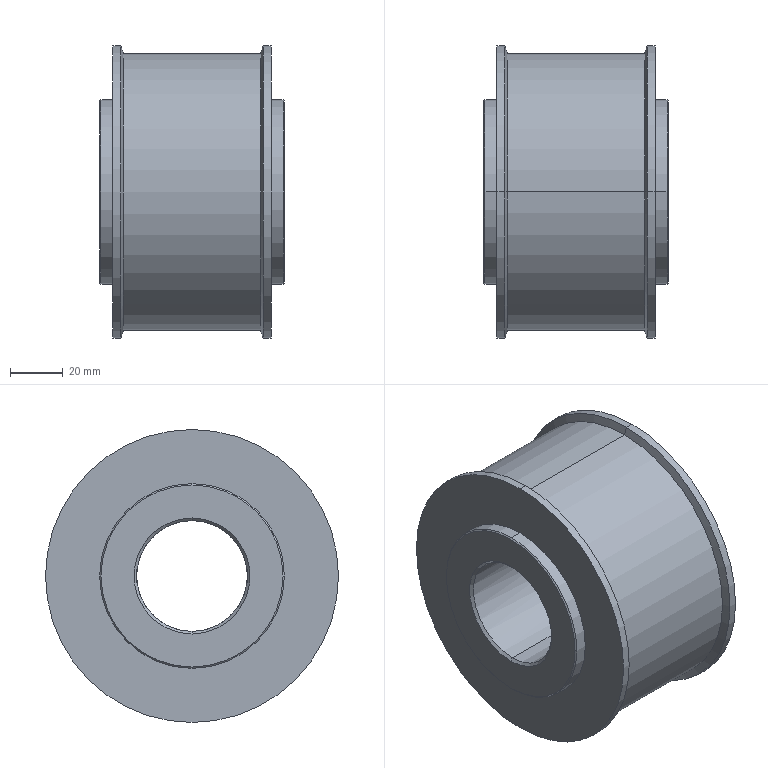Part | SolidWorks | features BaseBody 1 | 1 solid | 36 faces | box 70 x 111 x 111 mm | volume 426027 mm3 | cylinder 16 | cone 14 | plane 6 | commonest cylinder face diameters 70 x4 111 x4 42 x2 52 x2 62 x2 105 x2
STEP:
#1=CARTESIAN_POINT('',(-26.,0.,-52.5));
#2=VERTEX_POINT('',#1);
#3=CARTESIAN_POINT('',(-26.,0.,52.5));
#4=VERTEX_POINT('',#3);
#5=CARTESIAN_POINT('',(-26.,0.,0.));
#6=DIRECTION('',(1.,0.,0.));
#7=DIRECTION('',(0.,0.,-1.));
#8=AXIS2_PLACEMENT_3D('',#5,#6,#7);
#9=CIRCLE('',#8,52.5);
#10=EDGE_CURVE('',#2,#4,#9,.T.);
#11=ORIENTED_EDGE('',*,*,#10,.T.);
#12=CARTESIAN_POINT('',(26.,0.,52.5));
#13=VERTEX_POINT('',#12);
#14=CARTESIAN_POINT('',(-38.5,0.,52.5));
#15=DIRECTION('',(1.,0.,0.));
#16=VECTOR('',#15,1000.);
#17=LINE('',#14,#16);
#18=EDGE_CURVE('',#4,#13,#17,.T.);
#19=ORIENTED_EDGE('',*,*,#18,.T.);
#20=CARTESIAN_POINT('',(26.,0.,-52.5));
#21=VERTEX_POINT('',#20);
#22=CARTESIAN_POINT('',(26.,0.,0.));
#23=DIRECTION('',(-1.,0.,0.));
#24=DIRECTION('',(0.,0.,-1.));
#25=AXIS2_PLACEMENT_3D('',#22,#23,#24);
#26=CIRCLE('',#25,52.5);
#27=EDGE_CURVE('',#13,#21,#26,.T.);
#28=ORIENTED_EDGE('',*,*,#27,.T.);
#29=CARTESIAN_POINT('',(-38.5,0.,-52.5));
#30=DIRECTION('',(1.,0.,0.));
#31=VECTOR('',#30,1000.);
#32=LINE('',#29,#31);
#33=EDGE_CURVE('',#2,#21,#32,.T.);
#34=ORIENTED_EDGE('',*,*,#33,.F.);
#35=EDGE_LOOP('',(#11,#19,#28,#34));
#36=FACE_OUTER_BOUND('',#35,.T.);
#37=CARTESIAN_POINT('',(-38.5,0.,0.));
#38=DIRECTION('',(1.,0.,0.));
#39=DIRECTION('',(0.,0.,-1.));
#40=AXIS2_PLACEMENT_3D('',#37,#38,#39);
#41=CYLINDRICAL_SURFACE('',#40,52.5);
#42=ADVANCED_FACE('',(#36),#41,.T.);
#43=ORIENTED_EDGE('',*,*,#27,.F.);
#44=CARTESIAN_POINT('',(27.,0.,55.5));
#45=VERTEX_POINT('',#44);
#46=CARTESIAN_POINT('',(27.,0.,55.5));
#47=DIRECTION('',(0.3162,0.,0.9487));
#48=VECTOR('',#47,1000.);
#49=LINE('',#46,#48);
#50=EDGE_CURVE('',#13,#45,#49,.T.);
#51=ORIENTED_EDGE('',*,*,#50,.T.);
#52=CARTESIAN_POINT('',(27.,0.,-55.5));
#53=VERTEX_POINT('',#52);
#54=CARTESIAN_POINT('',(27.,0.,0.));
#55=DIRECTION('',(-1.,0.,0.));
#56=DIRECTION('',(0.,0.,1.));
#57=AXIS2_PLACEMENT_3D('',#54,#55,#56);
#58=CIRCLE('',#57,55.5);
#59=EDGE_CURVE('',#45,#53,#58,.T.);
#60=ORIENTED_EDGE('',*,*,#59,.T.);
#61=CARTESIAN_POINT('',(27.,0.,-55.5));
#62=DIRECTION('',(0.3162,0.,-0.9487));
#63=VECTOR('',#62,1000.);
#64=LINE('',#61,#63);
#65=EDGE_CURVE('',#21,#53,#64,.T.);
#66=ORIENTED_EDGE('',*,*,#65,.F.);
#67=EDGE_LOOP('',(#43,#51,#60,#66));
#68=FACE_OUTER_BOUND('',#67,.T.);
#69=CARTESIAN_POINT('',(27.,0.,0.));
#70=DIRECTION('',(1.,0.,0.));
#71=DIRECTION('',(0.,0.,-1.));
#72=AXIS2_PLACEMENT_3D('',#69,#70,#71);
#73=CONICAL_SURFACE('',#72,55.5,1.249);
#74=ADVANCED_FACE('',(#68),#73,.T.);
#75=ORIENTED_EDGE('',*,*,#10,.F.);
#76=CARTESIAN_POINT('',(-27.,0.,-55.5));
#77=VERTEX_POINT('',#76);
#78=CARTESIAN_POINT('',(-27.,0.,-55.5));
#79=DIRECTION('',(-0.3162,0.,-0.9487));
#80=VECTOR('',#79,1000.);
#81=LINE('',#78,#80);
#82=EDGE_CURVE('',#2,#77,#81,.T.);
#83=ORIENTED_EDGE('',*,*,#82,.T.);
#84=CARTESIAN_POINT('',(-27.,0.,55.5));
#85=VERTEX_POINT('',#84);
#86=CARTESIAN_POINT('',(-27.,0.,0.));
#87=DIRECTION('',(1.,0.,0.));
#88=DIRECTION('',(0.,0.,-1.));
#89=AXIS2_PLACEMENT_3D('',#86,#87,#88);
#90=CIRCLE('',#89,55.5);
#91=EDGE_CURVE('',#77,#85,#90,.T.);
#92=ORIENTED_EDGE('',*,*,#91,.T.);
#93=CARTESIAN_POINT('',(-27.,0.,55.5));
#94=DIRECTION('',(-0.3162,0.,0.9487));
#95=VECTOR('',#94,1000.);
#96=LINE('',#93,#95);
#97=EDGE_CURVE('',#4,#85,#96,.T.);
#98=ORIENTED_EDGE('',*,*,#97,.F.);
#99=EDGE_LOOP('',(#75,#83,#92,#98));
#100=FACE_OUTER_BOUND('',#99,.T.);
#101=CARTESIAN_POINT('',(-27.,0.,0.));
#102=DIRECTION('',(-1.,0.,0.));
#103=DIRECTION('',(0.,0.,1.));
#104=AXIS2_PLACEMENT_3D('',#101,#102,#103);
#105=CONICAL_SURFACE('',#104,55.5,1.249);
#106=ADVANCED_FACE('',(#100),#105,.T.);
#107=ORIENTED_EDGE('',*,*,#59,.F.);
#108=CARTESIAN_POINT('',(30.,0.,55.5));
#109=VERTEX_POINT('',#108);
#110=CARTESIAN_POINT('',(-38.5,0.,55.5));
#111=DIRECTION('',(1.,0.,0.));
#112=VECTOR('',#111,1000.);
#113=LINE('',#110,#112);
#114=EDGE_CURVE('',#45,#109,#113,.T.);
#115=ORIENTED_EDGE('',*,*,#114,.T.);
#116=CARTESIAN_POINT('',(30.,0.,-55.5));
#117=VERTEX_POINT('',#116);
#118=CARTESIAN_POINT('',(30.,0.,0.));
#119=DIRECTION('',(-1.,0.,0.));
#120=DIRECTION('',(0.,0.,-1.));
#121=AXIS2_PLACEMENT_3D('',#118,#119,#120);
#122=CIRCLE('',#121,55.5);
#123=EDGE_CURVE('',#109,#117,#122,.T.);
#124=ORIENTED_EDGE('',*,*,#123,.T.);
#125=CARTESIAN_POINT('',(-38.5,0.,-55.5));
#126=DIRECTION('',(1.,0.,0.));
#127=VECTOR('',#126,1000.);
#128=LINE('',#125,#127);
#129=EDGE_CURVE('',#53,#117,#128,.T.);
#130=ORIENTED_EDGE('',*,*,#129,.F.);
#131=EDGE_LOOP('',(#107,#115,#124,#130));
#132=FACE_OUTER_BOUND('',#131,.T.);
#133=CARTESIAN_POINT('',(-38.5,0.,0.));
#134=DIRECTION('',(1.,0.,0.));
#135=DIRECTION('',(0.,0.,-1.));
#136=AXIS2_PLACEMENT_3D('',#133,#134,#135);
#137=CYLINDRICAL_SURFACE('',#136,55.5);
#138=ADVANCED_FACE('',(#132),#137,.T.);
#139=CARTESIAN_POINT('',(-30.,0.,-55.5));
#140=VERTEX_POINT('',#139);
#141=CARTESIAN_POINT('',(-30.,0.,55.5));
#142=VERTEX_POINT('',#141);
#143=CARTESIAN_POINT('',(-30.,0.,0.));
#144=DIRECTION('',(1.,0.,0.));
#145=DIRECTION('',(0.,0.,-1.));
#146=AXIS2_PLACEMENT_3D('',#143,#144,#145);
#147=CIRCLE('',#146,55.5);
#148=EDGE_CURVE('',#140,#142,#147,.T.);
#149=ORIENTED_EDGE('',*,*,#148,.T.);
#150=CARTESIAN_POINT('',(-38.5,0.,55.5));
#151=DIRECTION('',(1.,0.,0.));
#152=VECTOR('',#151,1000.);
#153=LINE('',#150,#152);
#154=EDGE_CURVE('',#142,#85,#153,.T.);
#155=ORIENTED_EDGE('',*,*,#154,.T.);
#156=ORIENTED_EDGE('',*,*,#91,.F.);
#157=CARTESIAN_POINT('',(-38.5,0.,-55.5));
#158=DIRECTION('',(1.,0.,0.));
#159=VECTOR('',#158,1000.);
#160=LINE('',#157,#159);
#161=EDGE_CURVE('',#140,#77,#160,.T.);
#162=ORIENTED_EDGE('',*,*,#161,.F.);
#163=EDGE_LOOP('',(#149,#155,#156,#162));
#164=FACE_OUTER_BOUND('',#163,.T.);
#165=CARTESIAN_POINT('',(-38.5,0.,0.));
#166=DIRECTION('',(1.,0.,0.));
#167=DIRECTION('',(0.,0.,-1.));
#168=AXIS2_PLACEMENT_3D('',#165,#166,#167);
#169=CYLINDRICAL_SURFACE('',#168,55.5);
#170=ADVANCED_FACE('',(#164),#169,.T.);
#171=CARTESIAN_POINT('',(30.,0.,35.));
#172=VERTEX_POINT('',#171);
#173=CARTESIAN_POINT('',(30.,0.,-35.));
#174=VERTEX_POINT('',#173);
#175=CARTESIAN_POINT('',(30.,0.,0.));
#176=DIRECTION('',(-1.,0.,0.));
#177=DIRECTION('',(0.,0.,-1.));
#178=AXIS2_PLACEMENT_3D('',#175,#176,#177);
#179=CIRCLE('',#178,35.);
#180=EDGE_CURVE('',#172,#174,#179,.T.);
#181=ORIENTED_EDGE('',*,*,#180,.F.);
#182=CARTESIAN_POINT('',(34.5,0.,35.));
#183=VERTEX_POINT('',#182);
#184=CARTESIAN_POINT('',(-38.5,0.,35.));
#185=DIRECTION('',(1.,0.,0.));
#186=VECTOR('',#185,1000.);
#187=LINE('',#184,#186);
#188=EDGE_CURVE('',#172,#183,#187,.T.);
#189=ORIENTED_EDGE('',*,*,#188,.T.);
#190=CARTESIAN_POINT('',(34.5,0.,-35.));
#191=VERTEX_POINT('',#190);
#192=CARTESIAN_POINT('',(34.5,0.,0.));
#193=DIRECTION('',(-1.,0.,0.));
#194=DIRECTION('',(0.,0.,-1.));
#195=AXIS2_PLACEMENT_3D('',#192,#193,#194);
#196=CIRCLE('',#195,35.);
#197=EDGE_CURVE('',#183,#191,#196,.T.);
#198=ORIENTED_EDGE('',*,*,#197,.T.);
#199=CARTESIAN_POINT('',(-38.5,0.,-35.));
#200=DIRECTION('',(1.,0.,0.));
#201=VECTOR('',#200,1000.);
#202=LINE('',#199,#201);
#203=EDGE_CURVE('',#174,#191,#202,.T.);
#204=ORIENTED_EDGE('',*,*,#203,.F.);
#205=EDGE_LOOP('',(#181,#189,#198,#204));
#206=FACE_OUTER_BOUND('',#205,.T.);
#207=CARTESIAN_POINT('',(-38.5,0.,0.));
#208=DIRECTION('',(1.,0.,0.));
#209=DIRECTION('',(0.,0.,-1.));
#210=AXIS2_PLACEMENT_3D('',#207,#208,#209);
#211=CYLINDRICAL_SURFACE('',#210,35.);
#212=ADVANCED_FACE('',(#206),#211,.T.);
#213=CARTESIAN_POINT('',(-34.5,0.,-35.));
#214=VERTEX_POINT('',#213);
#215=CARTESIAN_POINT('',(-34.5,0.,35.));
#216=VERTEX_POINT('',#215);
#217=CARTESIAN_POINT('',(-34.5,0.,0.));
#218=DIRECTION('',(1.,0.,0.));
#219=DIRECTION('',(0.,0.,-1.));
#220=AXIS2_PLACEMENT_3D('',#217,#218,#219);
#221=CIRCLE('',#220,35.);
#222=EDGE_CURVE('',#214,#216,#221,.T.);
#223=ORIENTED_EDGE('',*,*,#222,.T.);
#224=CARTESIAN_POINT('',(-30.,0.,35.));
#225=VERTEX_POINT('',#224);
#226=CARTESIAN_POINT('',(-38.5,0.,35.));
#227=DIRECTION('',(1.,0.,0.));
#228=VECTOR('',#227,1000.);
#229=LINE('',#226,#228);
#230=EDGE_CURVE('',#216,#225,#229,.T.);
#231=ORIENTED_EDGE('',*,*,#230,.T.);
#232=CARTESIAN_POINT('',(-30.,0.,-35.));
#233=VERTEX_POINT('',#232);
#234=CARTESIAN_POINT('',(-30.,0.,0.));
#235=DIRECTION('',(-1.,0.,0.));
#236=DIRECTION('',(0.,0.,-1.));
#237=AXIS2_PLACEMENT_3D('',#234,#235,#236);
#238=CIRCLE('',#237,35.);
#239=EDGE_CURVE('',#225,#233,#238,.T.);
#240=ORIENTED_EDGE('',*,*,#239,.T.);
#241=CARTESIAN_POINT('',(-38.5,0.,-35.));
#242=DIRECTION('',(1.,0.,0.));
#243=VECTOR('',#242,1000.);
#244=LINE('',#241,#243);
#245=EDGE_CURVE('',#214,#233,#244,.T.);
#246=ORIENTED_EDGE('',*,*,#245,.F.);
#247=EDGE_LOOP('',(#223,#231,#240,#246));
#248=FACE_OUTER_BOUND('',#247,.T.);
#249=CARTESIAN_POINT('',(-38.5,0.,0.));
#250=DIRECTION('',(1.,0.,0.));
#251=DIRECTION('',(0.,0.,-1.));
#252=AXIS2_PLACEMENT_3D('',#249,#250,#251);
#253=CYLINDRICAL_SURFACE('',#252,35.);
#254=ADVANCED_FACE('',(#248),#253,.T.);
#255=CARTESIAN_POINT('',(35.,0.,34.5));
#256=VERTEX_POINT('',#255);
#257=CARTESIAN_POINT('',(35.,0.,-34.5));
#258=VERTEX_POINT('',#257);
#259=CARTESIAN_POINT('',(35.,0.,0.));
#260=DIRECTION('',(-1.,0.,0.));
#261=DIRECTION('',(0.,0.,1.));
#262=AXIS2_PLACEMENT_3D('',#259,#260,#261);
#263=CIRCLE('',#262,34.5);
#264=EDGE_CURVE('',#256,#258,#263,.T.);
#265=ORIENTED_EDGE('',*,*,#264,.T.);
#266=CARTESIAN_POINT('',(34.5,0.,-35.));
#267=DIRECTION('',(-0.7071,0.,-0.7071));
#268=VECTOR('',#267,1000.);
#269=LINE('',#266,#268);
#270=EDGE_CURVE('',#258,#191,#269,.T.);
#271=ORIENTED_EDGE('',*,*,#270,.T.);
#272=ORIENTED_EDGE('',*,*,#197,.F.);
#273=CARTESIAN_POINT('',(34.5,0.,35.));
#274=DIRECTION('',(-0.7071,0.,0.7071));
#275=VECTOR('',#274,1000.);
#276=LINE('',#273,#275);
#277=EDGE_CURVE('',#256,#183,#276,.T.);
#278=ORIENTED_EDGE('',*,*,#277,.F.);
#279=EDGE_LOOP('',(#265,#271,#272,#278));
#280=FACE_OUTER_BOUND('',#279,.T.);
#281=CARTESIAN_POINT('',(34.5,0.,0.));
#282=DIRECTION('',(-1.,0.,0.));
#283=DIRECTION('',(0.,0.,1.));
#284=AXIS2_PLACEMENT_3D('',#281,#282,#283);
#285=CONICAL_SURFACE('',#284,35.,0.7854);
#286=ADVANCED_FACE('',(#280),#285,.T.);
#287=CARTESIAN_POINT('',(-35.,0.,-34.5));
#288=VERTEX_POINT('',#287);
#289=CARTESIAN_POINT('',(-35.,0.,34.5));
#290=VERTEX_POINT('',#289);
#291=CARTESIAN_POINT('',(-35.,0.,0.));
#292=DIRECTION('',(1.,0.,0.));
#293=DIRECTION('',(0.,0.,-1.));
#294=AXIS2_PLACEMENT_3D('',#291,#292,#293);
#295=CIRCLE('',#294,34.5);
#296=EDGE_CURVE('',#288,#290,#295,.T.);
#297=ORIENTED_EDGE('',*,*,#296,.T.);
#298=CARTESIAN_POINT('',(-34.5,0.,35.));
#299=DIRECTION('',(0.7071,0.,0.7071));
#300=VECTOR('',#299,1000.);
#301=LINE('',#298,#300);
#302=EDGE_CURVE('',#290,#216,#301,.T.);
#303=ORIENTED_EDGE('',*,*,#302,.T.);
#304=ORIENTED_EDGE('',*,*,#222,.F.);
#305=CARTESIAN_POINT('',(-34.5,0.,-35.));
#306=DIRECTION('',(0.7071,0.,-0.7071));
#307=VECTOR('',#306,1000.);
#308=LINE('',#305,#307);
#309=EDGE_CURVE('',#288,#214,#308,.T.);
#310=ORIENTED_EDGE('',*,*,#309,.F.);
#311=EDGE_LOOP('',(#297,#303,#304,#310));
#312=FACE_OUTER_BOUND('',#311,.T.);
#313=CARTESIAN_POINT('',(-34.5,0.,0.));
#314=DIRECTION('',(1.,0.,0.));
#315=DIRECTION('',(0.,0.,-1.));
#316=AXIS2_PLACEMENT_3D('',#313,#314,#315);
#317=CONICAL_SURFACE('',#316,35.,0.7854);
#318=ADVANCED_FACE('',(#312),#317,.T.);
#319=CARTESIAN_POINT('',(34.,0.,31.));
#320=VERTEX_POINT('',#319);
#321=CARTESIAN_POINT('',(34.,0.,-31.));
#322=VERTEX_POINT('',#321);
#323=CARTESIAN_POINT('',(34.,0.,0.));
#324=DIRECTION('',(1.,0.,0.));
#325=DIRECTION('',(0.,0.,-1.));
#326=AXIS2_PLACEMENT_3D('',#323,#324,#325);
#327=CIRCLE('',#326,31.);
#328=EDGE_CURVE('',#320,#322,#327,.T.);
#329=ORIENTED_EDGE('',*,*,#328,.F.);
#330=CARTESIAN_POINT('',(35.,0.,32.));
#331=VERTEX_POINT('',#330);
#332=CARTESIAN_POINT('',(35.,0.,32.));
#333=DIRECTION('',(0.7071,0.,0.7071));
#334=VECTOR('',#333,1000.);
#335=LINE('',#332,#334);
#336=EDGE_CURVE('',#320,#331,#335,.T.);
#337=ORIENTED_EDGE('',*,*,#336,.T.);
#338=CARTESIAN_POINT('',(35.,0.,-32.));
#339=VERTEX_POINT('',#338);
#340=CARTESIAN_POINT('',(35.,0.,0.));
#341=DIRECTION('',(-1.,0.,0.));
#342=DIRECTION('',(0.,0.,-1.));
#343=AXIS2_PLACEMENT_3D('',#340,#341,#342);
#344=CIRCLE('',#343,32.);
#345=EDGE_CURVE('',#339,#331,#344,.T.);
#346=ORIENTED_EDGE('',*,*,#345,.F.);
#347=CARTESIAN_POINT('',(35.,0.,-32.));
#348=DIRECTION('',(0.7071,0.,-0.7071));
#349=VECTOR('',#348,1000.);
#350=LINE('',#347,#349);
#351=EDGE_CURVE('',#322,#339,#350,.T.);
#352=ORIENTED_EDGE('',*,*,#351,.F.);
#353=EDGE_LOOP('',(#329,#337,#346,#352));
#354=FACE_OUTER_BOUND('',#353,.T.);
#355=CARTESIAN_POINT('',(35.,0.,0.));
#356=DIRECTION('',(1.,0.,0.));
#357=DIRECTION('',(0.,0.,-1.));
#358=AXIS2_PLACEMENT_3D('',#355,#356,#357);
#359=CONICAL_SURFACE('',#358,32.,0.7854);
#360=ADVANCED_FACE('',(#354),#359,.F.);
#361=CARTESIAN_POINT('',(-34.,0.,-21.));
#362=VERTEX_POINT('',#361);
#363=CARTESIAN_POINT('',(-34.,0.,21.));
#364=VERTEX_POINT('',#363);
#365=CARTESIAN_POINT('',(-34.,0.,0.));
#366=DIRECTION('',(-1.,0.,0.));
#367=DIRECTION('',(0.,0.,-1.));
#368=AXIS2_PLACEMENT_3D('',#365,#366,#367);
#369=CIRCLE('',#368,21.);
#370=EDGE_CURVE('',#362,#364,#369,.T.);
#371=ORIENTED_EDGE('',*,*,#370,.F.);
#372=CARTESIAN_POINT('',(-35.,0.,-22.));
#373=VERTEX_POINT('',#372);
#374=CARTESIAN_POINT('',(-35.,0.,-22.));
#375=DIRECTION('',(-0.7071,0.,-0.7071));
#376=VECTOR('',#375,1000.);
#377=LINE('',#374,#376);
#378=EDGE_CURVE('',#362,#373,#377,.T.);
#379=ORIENTED_EDGE('',*,*,#378,.T.);
#380=CARTESIAN_POINT('',(-35.,0.,22.));
#381=VERTEX_POINT('',#380);
#382=CARTESIAN_POINT('',(-35.,0.,0.));
#383=DIRECTION('',(-1.,0.,0.));
#384=DIRECTION('',(0.,0.,1.));
#385=AXIS2_PLACEMENT_3D('',#382,#383,#384);
#386=CIRCLE('',#385,22.);
#387=EDGE_CURVE('',#373,#381,#386,.T.);
#388=ORIENTED_EDGE('',*,*,#387,.T.);
#389=CARTESIAN_POINT('',(-35.,0.,22.));
#390=DIRECTION('',(-0.7071,0.,0.7071));
#391=VECTOR('',#390,1000.);
#392=LINE('',#389,#391);
#393=EDGE_CURVE('',#364,#381,#392,.T.);
#394=ORIENTED_EDGE('',*,*,#393,.F.);
#395=EDGE_LOOP('',(#371,#379,#388,#394));
#396=FACE_OUTER_BOUND('',#395,.T.);
#397=CARTESIAN_POINT('',(-35.,0.,0.));
#398=DIRECTION('',(-1.,0.,0.));
#399=DIRECTION('',(0.,0.,1.));
#400=AXIS2_PLACEMENT_3D('',#397,#398,#399);
#401=CONICAL_SURFACE('',#400,22.,0.7854);
#402=ADVANCED_FACE('',(#396),#401,.F.);
#403=CARTESIAN_POINT('',(13.,0.,31.));
#404=VERTEX_POINT('',#403);
#405=CARTESIAN_POINT('',(13.,0.,-31.));
#406=VERTEX_POINT('',#405);
#407=CARTESIAN_POINT('',(13.,0.,0.));
#408=DIRECTION('',(1.,0.,0.));
#409=DIRECTION('',(0.,0.,-1.));
#410=AXIS2_PLACEMENT_3D('',#407,#408,#409);
#411=CIRCLE('',#410,31.);
#412=EDGE_CURVE('',#404,#406,#411,.T.);
#413=ORIENTED_EDGE('',*,*,#412,.F.);
#414=CARTESIAN_POINT('',(-38.5,0.,31.));
#415=DIRECTION('',(1.,0.,0.));
#416=VECTOR('',#415,1000.);
#417=LINE('',#414,#416);
#418=EDGE_CURVE('',#404,#320,#417,.T.);
#419=ORIENTED_EDGE('',*,*,#418,.T.);
#420=ORIENTED_EDGE('',*,*,#328,.T.);
#421=CARTESIAN_POINT('',(-38.5,0.,-31.));
#422=DIRECTION('',(1.,0.,0.));
#423=VECTOR('',#422,1000.);
#424=LINE('',#421,#423);
#425=EDGE_CURVE('',#406,#322,#424,.T.);
#426=ORIENTED_EDGE('',*,*,#425,.F.);
#427=EDGE_LOOP('',(#413,#419,#420,#426));
#428=FACE_OUTER_BOUND('',#427,.T.);
#429=CARTESIAN_POINT('',(-38.5,0.,0.));
#430=DIRECTION('',(1.,0.,0.));
#431=DIRECTION('',(0.,0.,-1.));
#432=AXIS2_PLACEMENT_3D('',#429,#430,#431);
#433=CYLINDRICAL_SURFACE('',#432,31.);
#434=ADVANCED_FACE('',(#428),#433,.F.);
#435=ORIENTED_EDGE('',*,*,#370,.T.);
#436=CARTESIAN_POINT('',(4.,0.,21.));
#437=VERTEX_POINT('',#436);
#438=CARTESIAN_POINT('',(-38.5,0.,21.));
#439=DIRECTION('',(1.,0.,0.));
#440=VECTOR('',#439,1000.);
#441=LINE('',#438,#440);
#442=EDGE_CURVE('',#364,#437,#441,.T.);
#443=ORIENTED_EDGE('',*,*,#442,.T.);
#444=CARTESIAN_POINT('',(4.,-21.,0.));
#445=VERTEX_POINT('',#444);
#446=CARTESIAN_POINT('',(4.,0.,0.));
#447=DIRECTION('',(-1.,0.,0.));
#448=DIRECTION('',(0.,0.,-1.));
#449=AXIS2_PLACEMENT_3D('',#446,#447,#448);
#450=CIRCLE('',#449,21.);
#451=EDGE_CURVE('',#445,#437,#450,.T.);
#452=ORIENTED_EDGE('',*,*,#451,.F.);
#453=CARTESIAN_POINT('',(4.,0.,-21.));
#454=VERTEX_POINT('',#453);
#455=CARTESIAN_POINT('',(4.,0.,0.));
#456=DIRECTION('',(-1.,0.,0.));
#457=DIRECTION('',(0.,0.,-1.));
#458=AXIS2_PLACEMENT_3D('',#455,#456,#457);
#459=CIRCLE('',#458,21.);
#460=EDGE_CURVE('',#454,#445,#459,.T.);
#461=ORIENTED_EDGE('',*,*,#460,.F.);
#462=CARTESIAN_POINT('',(-38.5,0.,-21.));
#463=DIRECTION('',(1.,0.,0.));
#464=VECTOR('',#463,1000.);
#465=LINE('',#462,#464);
#466=EDGE_CURVE('',#362,#454,#465,.T.);
#467=ORIENTED_EDGE('',*,*,#466,.F.);
#468=EDGE_LOOP('',(#435,#443,#452,#461,#467));
#469=FACE_OUTER_BOUND('',#468,.T.);
#470=CARTESIAN_POINT('',(-38.5,0.,0.));
#471=DIRECTION('',(1.,0.,0.));
#472=DIRECTION('',(0.,0.,-1.));
#473=AXIS2_PLACEMENT_3D('',#470,#471,#472);
#474=CYLINDRICAL_SURFACE('',#473,21.);
#475=ADVANCED_FACE('',(#469),#474,.F.);
#476=CARTESIAN_POINT('',(4.,21.,0.));
#477=VERTEX_POINT('',#476);
#478=CARTESIAN_POINT('',(4.,0.,0.));
#479=DIRECTION('',(-1.,0.,0.));
#480=DIRECTION('',(0.,0.,-1.));
#481=AXIS2_PLACEMENT_3D('',#478,#479,#480);
#482=CIRCLE('',#481,21.);
#483=EDGE_CURVE('',#477,#454,#482,.T.);
#484=ORIENTED_EDGE('',*,*,#483,.T.);
#485=ORIENTED_EDGE('',*,*,#460,.T.);
#486=CARTESIAN_POINT('',(5.,-22.,0.));
#487=VERTEX_POINT('',#486);
#488=CARTESIAN_POINT('',(5.,-22.,0.));
#489=DIRECTION('',(0.7071,-0.7071,0.));
#490=VECTOR('',#489,1000.);
#491=LINE('',#488,#490);
#492=EDGE_CURVE('',#445,#487,#491,.T.);
#493=ORIENTED_EDGE('',*,*,#492,.T.);
#494=CARTESIAN_POINT('',(5.,22.,0.));
#495=VERTEX_POINT('',#494);
#496=CARTESIAN_POINT('',(5.,0.,0.));
#497=DIRECTION('',(-1.,0.,0.));
#498=DIRECTION('',(0.,1.,0.));
#499=AXIS2_PLACEMENT_3D('',#496,#497,#498);
#500=CIRCLE('',#499,22.);
#501=EDGE_CURVE('',#495,#487,#500,.T.);
#502=ORIENTED_EDGE('',*,*,#501,.F.);
#503=CARTESIAN_POINT('',(5.,22.,0.));
#504=DIRECTION('',(0.7071,0.7071,0.));
#505=VECTOR('',#504,1000.);
#506=LINE('',#503,#505);
#507=EDGE_CURVE('',#477,#495,#506,.T.);
#508=ORIENTED_EDGE('',*,*,#507,.F.);
#509=EDGE_LOOP('',(#484,#485,#493,#502,#508));
#510=FACE_OUTER_BOUND('',#509,.T.);
#511=CARTESIAN_POINT('',(5.,0.,0.));
#512=DIRECTION('',(1.,0.,0.));
#513=DIRECTION('',(0.,1.,0.));
#514=AXIS2_PLACEMENT_3D('',#511,#512,#513);
#515=CONICAL_SURFACE('',#514,22.,0.7854);
#516=ADVANCED_FACE('',(#510),#515,.F.);
#517=CARTESIAN_POINT('',(5.,0.,26.));
#518=VERTEX_POINT('',#517);
#519=CARTESIAN_POINT('',(5.,0.,-26.));
#520=VERTEX_POINT('',#519);
#521=CARTESIAN_POINT('',(5.,0.,0.));
#522=DIRECTION('',(1.,0.,0.));
#523=DIRECTION('',(0.,0.,-1.));
#524=AXIS2_PLACEMENT_3D('',#521,#522,#523);
#525=CIRCLE('',#524,26.);
#526=EDGE_CURVE('',#518,#520,#525,.T.);
#527=ORIENTED_EDGE('',*,*,#526,.F.);
#528=CARTESIAN_POINT('',(13.,0.,26.));
#529=VERTEX_POINT('',#528);
#530=CARTESIAN_POINT('',(-38.5,0.,26.));
#531=DIRECTION('',(1.,0.,0.));
#532=VECTOR('',#531,1000.);
#533=LINE('',#530,#532);
#534=EDGE_CURVE('',#518,#529,#533,.T.);
#535=ORIENTED_EDGE('',*,*,#534,.T.);
#536=CARTESIAN_POINT('',(13.,0.,-26.));
#537=VERTEX_POINT('',#536);
#538=CARTESIAN_POINT('',(13.,0.,0.));
#539=DIRECTION('',(-1.,0.,0.));
#540=DIRECTION('',(0.,0.,-1.));
#541=AXIS2_PLACEMENT_3D('',#538,#539,#540);
#542=CIRCLE('',#541,26.);
#543=EDGE_CURVE('',#537,#529,#542,.T.);
#544=ORIENTED_EDGE('',*,*,#543,.F.);
#545=CARTESIAN_POINT('',(-38.5,0.,-26.));
#546=DIRECTION('',(1.,0.,0.));
#547=VECTOR('',#546,1000.);
#548=LINE('',#545,#547);
#549=EDGE_CURVE('',#520,#537,#548,.T.);
#550=ORIENTED_EDGE('',*,*,#549,.F.);
#551=EDGE_LOOP('',(#527,#535,#544,#550));
#552=FACE_OUTER_BOUND('',#551,.T.);
#553=CARTESIAN_POINT('',(-38.5,0.,0.));
#554=DIRECTION('',(1.,0.,0.));
#555=DIRECTION('',(0.,0.,-1.));
#556=AXIS2_PLACEMENT_3D('',#553,#554,#555);
#557=CYLINDRICAL_SURFACE('',#556,26.);
#558=ADVANCED_FACE('',(#552),#557,.F.);
#559=ORIENTED_EDGE('',*,*,#18,.F.);
#560=CARTESIAN_POINT('',(-26.,0.,0.));
#561=DIRECTION('',(1.,0.,0.));
#562=DIRECTION('',(0.,0.,-1.));
#563=AXIS2_PLACEMENT_3D('',#560,#561,#562);
#564=CIRCLE('',#563,52.5);
#565=EDGE_CURVE('',#4,#2,#564,.T.);
#566=ORIENTED_EDGE('',*,*,#565,.T.);
#567=ORIENTED_EDGE('',*,*,#33,.T.);
#568=CARTESIAN_POINT('',(26.,0.,0.));
#569=DIRECTION('',(-1.,0.,0.));
#570=DIRECTION('',(0.,0.,-1.));
#571=AXIS2_PLACEMENT_3D('',#568,#569,#570);
#572=CIRCLE('',#571,52.5);
#573=EDGE_CURVE('',#21,#13,#572,.T.);
#574=ORIENTED_EDGE('',*,*,#573,.T.);
#575=EDGE_LOOP('',(#559,#566,#567,#574));
#576=FACE_OUTER_BOUND('',#575,.T.);
#577=CARTESIAN_POINT('',(-38.5,0.,0.));
#578=DIRECTION('',(1.,0.,0.));
#579=DIRECTION('',(0.,0.,-1.));
#580=AXIS2_PLACEMENT_3D('',#577,#578,#579);
#581=CYLINDRICAL_SURFACE('',#580,52.5);
#582=ADVANCED_FACE('',(#576),#581,.T.);
#583=ORIENTED_EDGE('',*,*,#50,.F.);
#584=ORIENTED_EDGE('',*,*,#573,.F.);
#585=ORIENTED_EDGE('',*,*,#65,.T.);
#586=CARTESIAN_POINT('',(27.,0.,0.));
#587=DIRECTION('',(-1.,0.,0.));
#588=DIRECTION('',(0.,0.,1.));
#589=AXIS2_PLACEMENT_3D('',#586,#587,#588);
#590=CIRCLE('',#589,55.5);
#591=EDGE_CURVE('',#53,#45,#590,.T.);
#592=ORIENTED_EDGE('',*,*,#591,.T.);
#593=EDGE_LOOP('',(#583,#584,#585,#592));
#594=FACE_OUTER_BOUND('',#593,.T.);
#595=CARTESIAN_POINT('',(27.,0.,0.));
#596=DIRECTION('',(1.,0.,0.));
#597=DIRECTION('',(0.,0.,-1.));
#598=AXIS2_PLACEMENT_3D('',#595,#596,#597);
#599=CONICAL_SURFACE('',#598,55.5,1.249);
#600=ADVANCED_FACE('',(#594),#599,.T.);
#601=ORIENTED_EDGE('',*,*,#82,.F.);
#602=ORIENTED_EDGE('',*,*,#565,.F.);
#603=ORIENTED_EDGE('',*,*,#97,.T.);
#604=CARTESIAN_POINT('',(-27.,0.,0.));
#605=DIRECTION('',(1.,0.,0.));
#606=DIRECTION('',(0.,0.,-1.));
#607=AXIS2_PLACEMENT_3D('',#604,#605,#606);
#608=CIRCLE('',#607,55.5);
#609=EDGE_CURVE('',#85,#77,#608,.T.);
#610=ORIENTED_EDGE('',*,*,#609,.T.);
#611=EDGE_LOOP('',(#601,#602,#603,#610));
#612=FACE_OUTER_BOUND('',#611,.T.);
#613=CARTESIAN_POINT('',(-27.,0.,0.));
#614=DIRECTION('',(-1.,0.,0.));
#615=DIRECTION('',(0.,0.,1.));
#616=AXIS2_PLACEMENT_3D('',#613,#614,#615);
#617=CONICAL_SURFACE('',#616,55.5,1.249);
#618=ADVANCED_FACE('',(#612),#617,.T.);
#619=ORIENTED_EDGE('',*,*,#114,.F.);
#620=ORIENTED_EDGE('',*,*,#591,.F.);
#621=ORIENTED_EDGE('',*,*,#129,.T.);
#622=CARTESIAN_POINT('',(30.,0.,0.));
#623=DIRECTION('',(-1.,0.,0.));
#624=DIRECTION('',(0.,0.,-1.));
#625=AXIS2_PLACEMENT_3D('',#622,#623,#624);
#626=CIRCLE('',#625,55.5);
#627=EDGE_CURVE('',#117,#109,#626,.T.);
#628=ORIENTED_EDGE('',*,*,#627,.T.);
#629=EDGE_LOOP('',(#619,#620,#621,#628));
#630=FACE_OUTER_BOUND('',#629,.T.);
#631=CARTESIAN_POINT('',(-38.5,0.,0.));
#632=DIRECTION('',(1.,0.,0.));
#633=DIRECTION('',(0.,0.,-1.));
#634=AXIS2_PLACEMENT_3D('',#631,#632,#633);
#635=CYLINDRICAL_SURFACE('',#634,55.5);
#636=ADVANCED_FACE('',(#630),#635,.T.);
#637=ORIENTED_EDGE('',*,*,#154,.F.);
#638=CARTESIAN_POINT('',(-30.,0.,0.));
#639=DIRECTION('',(1.,0.,0.));
#640=DIRECTION('',(0.,0.,-1.));
#641=AXIS2_PLACEMENT_3D('',#638,#639,#640);
#642=CIRCLE('',#641,55.5);
#643=EDGE_CURVE('',#142,#140,#642,.T.);
#644=ORIENTED_EDGE('',*,*,#643,.T.);
#645=ORIENTED_EDGE('',*,*,#161,.T.);
#646=ORIENTED_EDGE('',*,*,#609,.F.);
#647=EDGE_LOOP('',(#637,#644,#645,#646));
#648=FACE_OUTER_BOUND('',#647,.T.);
#649=CARTESIAN_POINT('',(-38.5,0.,0.));
#650=DIRECTION('',(1.,0.,0.));
#651=DIRECTION('',(0.,0.,-1.));
#652=AXIS2_PLACEMENT_3D('',#649,#650,#651);
#653=CYLINDRICAL_SURFACE('',#652,55.5);
#654=ADVANCED_FACE('',(#648),#653,.T.);
#655=CARTESIAN_POINT('',(30.,0.,0.));
#656=DIRECTION('',(-1.,0.,0.));
#657=DIRECTION('',(0.,0.,-1.));
#658=AXIS2_PLACEMENT_3D('',#655,#656,#657);
#659=CIRCLE('',#658,35.);
#660=EDGE_CURVE('',#174,#172,#659,.T.);
#661=ORIENTED_EDGE('',*,*,#660,.T.);
#662=ORIENTED_EDGE('',*,*,#180,.T.);
#663=EDGE_LOOP('',(#661,#662));
#664=FACE_BOUND('',#663,.T.);
#665=ORIENTED_EDGE('',*,*,#627,.F.);
#666=ORIENTED_EDGE('',*,*,#123,.F.);
#667=EDGE_LOOP('',(#665,#666));
#668=FACE_OUTER_BOUND('',#667,.T.);
#669=CARTESIAN_POINT('',(30.,0.,0.));
#670=DIRECTION('',(1.,0.,0.));
#671=DIRECTION('',(0.,0.,-1.));
#672=AXIS2_PLACEMENT_3D('',#669,#670,#671);
#673=PLANE('',#672);
#674=ADVANCED_FACE('',(#664,#668),#673,.T.);
#675=CARTESIAN_POINT('',(-30.,0.,0.));
#676=DIRECTION('',(-1.,0.,0.));
#677=DIRECTION('',(0.,0.,-1.));
#678=AXIS2_PLACEMENT_3D('',#675,#676,#677);
#679=CIRCLE('',#678,35.);
#680=EDGE_CURVE('',#233,#225,#679,.T.);
#681=ORIENTED_EDGE('',*,*,#680,.F.);
#682=ORIENTED_EDGE('',*,*,#239,.F.);
#683=EDGE_LOOP('',(#681,#682));
#684=FACE_BOUND('',#683,.T.);
#685=ORIENTED_EDGE('',*,*,#148,.F.);
#686=ORIENTED_EDGE('',*,*,#643,.F.);
#687=EDGE_LOOP('',(#685,#686));
#688=FACE_OUTER_BOUND('',#687,.T.);
#689=CARTESIAN_POINT('',(-30.,0.,0.));
#690=DIRECTION('',(1.,0.,0.));
#691=DIRECTION('',(0.,0.,-1.));
#692=AXIS2_PLACEMENT_3D('',#689,#690,#691);
#693=PLANE('',#692);
#694=ADVANCED_FACE('',(#684,#688),#693,.F.);
#695=ORIENTED_EDGE('',*,*,#188,.F.);
#696=ORIENTED_EDGE('',*,*,#660,.F.);
#697=ORIENTED_EDGE('',*,*,#203,.T.);
#698=CARTESIAN_POINT('',(34.5,0.,0.));
#699=DIRECTION('',(-1.,0.,0.));
#700=DIRECTION('',(0.,0.,-1.));
#701=AXIS2_PLACEMENT_3D('',#698,#699,#700);
#702=CIRCLE('',#701,35.);
#703=EDGE_CURVE('',#191,#183,#702,.T.);
#704=ORIENTED_EDGE('',*,*,#703,.T.);
#705=EDGE_LOOP('',(#695,#696,#697,#704));
#706=FACE_OUTER_BOUND('',#705,.T.);
#707=CARTESIAN_POINT('',(-38.5,0.,0.));
#708=DIRECTION('',(1.,0.,0.));
#709=DIRECTION('',(0.,0.,-1.));
#710=AXIS2_PLACEMENT_3D('',#707,#708,#709);
#711=CYLINDRICAL_SURFACE('',#710,35.);
#712=ADVANCED_FACE('',(#706),#711,.T.);
#713=ORIENTED_EDGE('',*,*,#230,.F.);
#714=CARTESIAN_POINT('',(-34.5,0.,0.));
#715=DIRECTION('',(1.,0.,0.));
#716=DIRECTION('',(0.,0.,-1.));
#717=AXIS2_PLACEMENT_3D('',#714,#715,#716);
#718=CIRCLE('',#717,35.);
#719=EDGE_CURVE('',#216,#214,#718,.T.);
#720=ORIENTED_EDGE('',*,*,#719,.T.);
#721=ORIENTED_EDGE('',*,*,#245,.T.);
#722=ORIENTED_EDGE('',*,*,#680,.T.);
#723=EDGE_LOOP('',(#713,#720,#721,#722));
#724=FACE_OUTER_BOUND('',#723,.T.);
#725=CARTESIAN_POINT('',(-38.5,0.,0.));
#726=DIRECTION('',(1.,0.,0.));
#727=DIRECTION('',(0.,0.,-1.));
#728=AXIS2_PLACEMENT_3D('',#725,#726,#727);
#729=CYLINDRICAL_SURFACE('',#728,35.);
#730=ADVANCED_FACE('',(#724),#729,.T.);
#731=ORIENTED_EDGE('',*,*,#270,.F.);
#732=CARTESIAN_POINT('',(35.,0.,0.));
#733=DIRECTION('',(-1.,0.,0.));
#734=DIRECTION('',(0.,0.,1.));
#735=AXIS2_PLACEMENT_3D('',#732,#733,#734);
#736=CIRCLE('',#735,34.5);
#737=EDGE_CURVE('',#258,#256,#736,.T.);
#738=ORIENTED_EDGE('',*,*,#737,.T.);
#739=ORIENTED_EDGE('',*,*,#277,.T.);
#740=ORIENTED_EDGE('',*,*,#703,.F.);
#741=EDGE_LOOP('',(#731,#738,#739,#740));
#742=FACE_OUTER_BOUND('',#741,.T.);
#743=CARTESIAN_POINT('',(34.5,0.,0.));
#744=DIRECTION('',(-1.,0.,0.));
#745=DIRECTION('',(0.,0.,1.));
#746=AXIS2_PLACEMENT_3D('',#743,#744,#745);
#747=CONICAL_SURFACE('',#746,35.,0.7854);
#748=ADVANCED_FACE('',(#742),#747,.T.);
#749=ORIENTED_EDGE('',*,*,#302,.F.);
#750=CARTESIAN_POINT('',(-35.,0.,0.));
#751=DIRECTION('',(1.,0.,0.));
#752=DIRECTION('',(0.,0.,-1.));
#753=AXIS2_PLACEMENT_3D('',#750,#751,#752);
#754=CIRCLE('',#753,34.5);
#755=EDGE_CURVE('',#290,#288,#754,.T.);
#756=ORIENTED_EDGE('',*,*,#755,.T.);
#757=ORIENTED_EDGE('',*,*,#309,.T.);
#758=ORIENTED_EDGE('',*,*,#719,.F.);
#759=EDGE_LOOP('',(#749,#756,#757,#758));
#760=FACE_OUTER_BOUND('',#759,.T.);
#761=CARTESIAN_POINT('',(-34.5,0.,0.));
#762=DIRECTION('',(1.,0.,0.));
#763=DIRECTION('',(0.,0.,-1.));
#764=AXIS2_PLACEMENT_3D('',#761,#762,#763);
#765=CONICAL_SURFACE('',#764,35.,0.7854);
#766=ADVANCED_FACE('',(#760),#765,.T.);
#767=ORIENTED_EDGE('',*,*,#345,.T.);
#768=CARTESIAN_POINT('',(35.,0.,0.));
#769=DIRECTION('',(-1.,0.,0.));
#770=DIRECTION('',(0.,0.,-1.));
#771=AXIS2_PLACEMENT_3D('',#768,#769,#770);
#772=CIRCLE('',#771,32.);
#773=EDGE_CURVE('',#331,#339,#772,.T.);
#774=ORIENTED_EDGE('',*,*,#773,.T.);
#775=EDGE_LOOP('',(#767,#774));
#776=FACE_BOUND('',#775,.T.);
#777=ORIENTED_EDGE('',*,*,#264,.F.);
#778=ORIENTED_EDGE('',*,*,#737,.F.);
#779=EDGE_LOOP('',(#777,#778));
#780=FACE_OUTER_BOUND('',#779,.T.);
#781=CARTESIAN_POINT('',(35.,0.,0.));
#782=DIRECTION('',(1.,0.,0.));
#783=DIRECTION('',(0.,0.,-1.));
#784=AXIS2_PLACEMENT_3D('',#781,#782,#783);
#785=PLANE('',#784);
#786=ADVANCED_FACE('',(#776,#780),#785,.T.);
#787=CARTESIAN_POINT('',(-35.,0.,0.));
#788=DIRECTION('',(-1.,0.,0.));
#789=DIRECTION('',(0.,0.,1.));
#790=AXIS2_PLACEMENT_3D('',#787,#788,#789);
#791=CIRCLE('',#790,22.);
#792=EDGE_CURVE('',#381,#373,#791,.T.);
#793=ORIENTED_EDGE('',*,*,#792,.F.);
#794=ORIENTED_EDGE('',*,*,#387,.F.);
#795=EDGE_LOOP('',(#793,#794));
#796=FACE_BOUND('',#795,.T.);
#797=ORIENTED_EDGE('',*,*,#296,.F.);
#798=ORIENTED_EDGE('',*,*,#755,.F.);
#799=EDGE_LOOP('',(#797,#798));
#800=FACE_OUTER_BOUND('',#799,.T.);
#801=CARTESIAN_POINT('',(-35.,0.,0.));
#802=DIRECTION('',(1.,0.,0.));
#803=DIRECTION('',(0.,0.,-1.));
#804=AXIS2_PLACEMENT_3D('',#801,#802,#803);
#805=PLANE('',#804);
#806=ADVANCED_FACE('',(#796,#800),#805,.F.);
#807=ORIENTED_EDGE('',*,*,#336,.F.);
#808=CARTESIAN_POINT('',(34.,0.,0.));
#809=DIRECTION('',(1.,0.,0.));
#810=DIRECTION('',(0.,0.,-1.));
#811=AXIS2_PLACEMENT_3D('',#808,#809,#810);
#812=CIRCLE('',#811,31.);
#813=EDGE_CURVE('',#322,#320,#812,.T.);
#814=ORIENTED_EDGE('',*,*,#813,.F.);
#815=ORIENTED_EDGE('',*,*,#351,.T.);
#816=ORIENTED_EDGE('',*,*,#773,.F.);
#817=EDGE_LOOP('',(#807,#814,#815,#816));
#818=FACE_OUTER_BOUND('',#817,.T.);
#819=CARTESIAN_POINT('',(35.,0.,0.));
#820=DIRECTION('',(1.,0.,0.));
#821=DIRECTION('',(0.,0.,-1.));
#822=AXIS2_PLACEMENT_3D('',#819,#820,#821);
#823=CONICAL_SURFACE('',#822,32.,0.7854);
#824=ADVANCED_FACE('',(#818),#823,.F.);
#825=ORIENTED_EDGE('',*,*,#378,.F.);
#826=CARTESIAN_POINT('',(-34.,0.,0.));
#827=DIRECTION('',(-1.,0.,0.));
#828=DIRECTION('',(0.,0.,-1.));
#829=AXIS2_PLACEMENT_3D('',#826,#827,#828);
#830=CIRCLE('',#829,21.);
#831=EDGE_CURVE('',#364,#362,#830,.T.);
#832=ORIENTED_EDGE('',*,*,#831,.F.);
#833=ORIENTED_EDGE('',*,*,#393,.T.);
#834=ORIENTED_EDGE('',*,*,#792,.T.);
#835=EDGE_LOOP('',(#825,#832,#833,#834));
#836=FACE_OUTER_BOUND('',#835,.T.);
#837=CARTESIAN_POINT('',(-35.,0.,0.));
#838=DIRECTION('',(-1.,0.,0.));
#839=DIRECTION('',(0.,0.,1.));
#840=AXIS2_PLACEMENT_3D('',#837,#838,#839);
#841=CONICAL_SURFACE('',#840,22.,0.7854);
#842=ADVANCED_FACE('',(#836),#841,.F.);
#843=ORIENTED_EDGE('',*,*,#418,.F.);
#844=CARTESIAN_POINT('',(13.,0.,0.));
#845=DIRECTION('',(1.,0.,0.));
#846=DIRECTION('',(0.,0.,-1.));
#847=AXIS2_PLACEMENT_3D('',#844,#845,#846);
#848=CIRCLE('',#847,31.);
#849=EDGE_CURVE('',#406,#404,#848,.T.);
#850=ORIENTED_EDGE('',*,*,#849,.F.);
#851=ORIENTED_EDGE('',*,*,#425,.T.);
#852=ORIENTED_EDGE('',*,*,#813,.T.);
#853=EDGE_LOOP('',(#843,#850,#851,#852));
#854=FACE_OUTER_BOUND('',#853,.T.);
#855=CARTESIAN_POINT('',(-38.5,0.,0.));
#856=DIRECTION('',(1.,0.,0.));
#857=DIRECTION('',(0.,0.,-1.));
#858=AXIS2_PLACEMENT_3D('',#855,#856,#857);
#859=CYLINDRICAL_SURFACE('',#858,31.);
#860=ADVANCED_FACE('',(#854),#859,.F.);
#861=ORIENTED_EDGE('',*,*,#442,.F.);
#862=ORIENTED_EDGE('',*,*,#831,.T.);
#863=ORIENTED_EDGE('',*,*,#466,.T.);
#864=ORIENTED_EDGE('',*,*,#483,.F.);
#865=CARTESIAN_POINT('',(4.,0.,0.));
#866=DIRECTION('',(-1.,0.,0.));
#867=DIRECTION('',(0.,0.,-1.));
#868=AXIS2_PLACEMENT_3D('',#865,#866,#867);
#869=CIRCLE('',#868,21.);
#870=EDGE_CURVE('',#437,#477,#869,.T.);
#871=ORIENTED_EDGE('',*,*,#870,.F.);
#872=EDGE_LOOP('',(#861,#862,#863,#864,#871));
#873=FACE_OUTER_BOUND('',#872,.T.);
#874=CARTESIAN_POINT('',(-38.5,0.,0.));
#875=DIRECTION('',(1.,0.,0.));
#876=DIRECTION('',(0.,0.,-1.));
#877=AXIS2_PLACEMENT_3D('',#874,#875,#876);
#878=CYLINDRICAL_SURFACE('',#877,21.);
#879=ADVANCED_FACE('',(#873),#878,.F.);
#880=ORIENTED_EDGE('',*,*,#543,.T.);
#881=CARTESIAN_POINT('',(13.,0.,0.));
#882=DIRECTION('',(-1.,0.,0.));
#883=DIRECTION('',(0.,0.,-1.));
#884=AXIS2_PLACEMENT_3D('',#881,#882,#883);
#885=CIRCLE('',#884,26.);
#886=EDGE_CURVE('',#529,#537,#885,.T.);
#887=ORIENTED_EDGE('',*,*,#886,.T.);
#888=EDGE_LOOP('',(#880,#887));
#889=FACE_BOUND('',#888,.T.);
#890=ORIENTED_EDGE('',*,*,#849,.T.);
#891=ORIENTED_EDGE('',*,*,#412,.T.);
#892=EDGE_LOOP('',(#890,#891));
#893=FACE_OUTER_BOUND('',#892,.T.);
#894=CARTESIAN_POINT('',(13.,0.,0.));
#895=DIRECTION('',(1.,0.,0.));
#896=DIRECTION('',(0.,0.,-1.));
#897=AXIS2_PLACEMENT_3D('',#894,#895,#896);
#898=PLANE('',#897);
#899=ADVANCED_FACE('',(#889,#893),#898,.T.);
#900=ORIENTED_EDGE('',*,*,#492,.F.);
#901=ORIENTED_EDGE('',*,*,#451,.T.);
#902=ORIENTED_EDGE('',*,*,#870,.T.);
#903=ORIENTED_EDGE('',*,*,#507,.T.);
#904=CARTESIAN_POINT('',(5.,0.,0.));
#905=DIRECTION('',(-1.,0.,0.));
#906=DIRECTION('',(0.,1.,0.));
#907=AXIS2_PLACEMENT_3D('',#904,#905,#906);
#908=CIRCLE('',#907,22.);
#909=EDGE_CURVE('',#487,#495,#908,.T.);
#910=ORIENTED_EDGE('',*,*,#909,.F.);
#911=EDGE_LOOP('',(#900,#901,#902,#903,#910));
#912=FACE_OUTER_BOUND('',#911,.T.);
#913=CARTESIAN_POINT('',(5.,0.,0.));
#914=DIRECTION('',(1.,0.,0.));
#915=DIRECTION('',(0.,1.,0.));
#916=AXIS2_PLACEMENT_3D('',#913,#914,#915);
#917=CONICAL_SURFACE('',#916,22.,0.7854);
#918=ADVANCED_FACE('',(#912),#917,.F.);
#919=ORIENTED_EDGE('',*,*,#534,.F.);
#920=CARTESIAN_POINT('',(5.,0.,0.));
#921=DIRECTION('',(1.,0.,0.));
#922=DIRECTION('',(0.,0.,-1.));
#923=AXIS2_PLACEMENT_3D('',#920,#921,#922);
#924=CIRCLE('',#923,26.);
#925=EDGE_CURVE('',#520,#518,#924,.T.);
#926=ORIENTED_EDGE('',*,*,#925,.F.);
#927=ORIENTED_EDGE('',*,*,#549,.T.);
#928=ORIENTED_EDGE('',*,*,#886,.F.);
#929=EDGE_LOOP('',(#919,#926,#927,#928));
#930=FACE_OUTER_BOUND('',#929,.T.);
#931=CARTESIAN_POINT('',(-38.5,0.,0.));
#932=DIRECTION('',(1.,0.,0.));
#933=DIRECTION('',(0.,0.,-1.));
#934=AXIS2_PLACEMENT_3D('',#931,#932,#933);
#935=CYLINDRICAL_SURFACE('',#934,26.);
#936=ADVANCED_FACE('',(#930),#935,.F.);
#937=ORIENTED_EDGE('',*,*,#501,.T.);
#938=ORIENTED_EDGE('',*,*,#909,.T.);
#939=EDGE_LOOP('',(#937,#938));
#940=FACE_BOUND('',#939,.T.);
#941=ORIENTED_EDGE('',*,*,#925,.T.);
#942=ORIENTED_EDGE('',*,*,#526,.T.);
#943=EDGE_LOOP('',(#941,#942));
#944=FACE_OUTER_BOUND('',#943,.T.);
#945=CARTESIAN_POINT('',(5.,0.,0.));
#946=DIRECTION('',(1.,0.,0.));
#947=DIRECTION('',(0.,0.,-1.));
#948=AXIS2_PLACEMENT_3D('',#945,#946,#947);
#949=PLANE('',#948);
#950=ADVANCED_FACE('',(#940,#944),#949,.T.);
#951=CLOSED_SHELL('',(#42,#74,#106,#138,#170,#212,#254,#286,#318,#360,#402,#434,#475,#516,#558,#582,#600,#618,#636,#654,#674,#694,#712,#730,#748,#766,#786,#806,#824,#842,#860,#879,#899,#918,#936,#950));
#952=MANIFOLD_SOLID_BREP('',#951);
#953=CARTESIAN_POINT('',(0.,0.,0.));
#954=DIRECTION('',(0.,0.,1.));
#955=DIRECTION('',(1.,0.,0.));
#956=AXIS2_PLACEMENT_3D('',#953,#954,#955);
#957=(LENGTH_UNIT()NAMED_UNIT(*)SI_UNIT(.MILLI.,.METRE.));
#958=UNCERTAINTY_MEASURE_WITH_UNIT(LENGTH_MEASURE(0.00001),#957,'','');
#959=(NAMED_UNIT(*)PLANE_ANGLE_UNIT()SI_UNIT($,.RADIAN.));
#960=(NAMED_UNIT(*)SI_UNIT($,.STERADIAN.)SOLID_ANGLE_UNIT());
#961=(GEOMETRIC_REPRESENTATION_CONTEXT(3)GLOBAL_UNCERTAINTY_ASSIGNED_CONTEXT((#958))GLOBAL_UNIT_ASSIGNED_CONTEXT((#957,#959,#960))REPRESENTATION_CONTEXT('',''));
#962=ADVANCED_BREP_SHAPE_REPRESENTATION('',(#952,#956),#961);